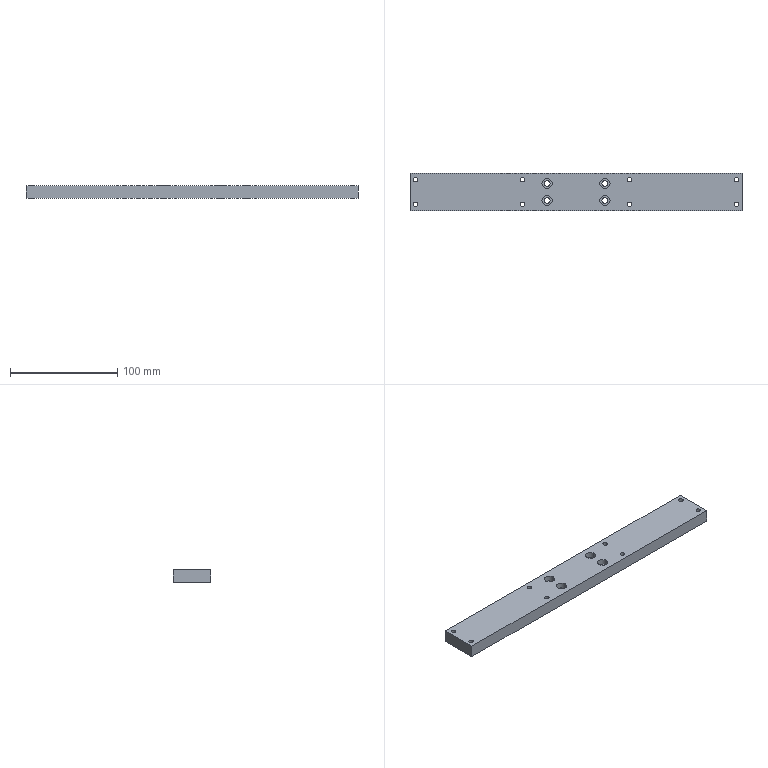Part | SolidWorks | features HoleWzd 3, Extrusion 1, LPattern 1 | 1 solid | 54 faces | box 310 x 35 x 12 mm | volume 126366 mm3 | cylinder 38 | plane 10 | cone 6 | commonest cylinder face diameters 4.2 x16 5.5 x8 9.5 x8 3.3 x6